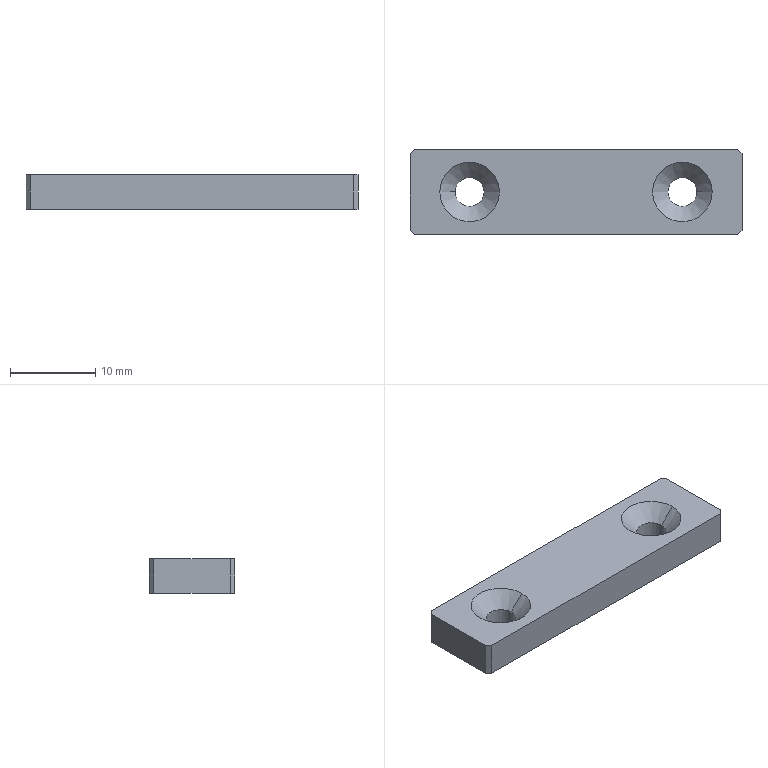Part | NX | features BREP 1 | 1 solid | 18 faces | box 39 x 10 x 4 mm | volume 1439 mm3 | plane 10 | cone 4 | cylinder 4 | commonest cylinder face diameters 3.4 x4
STEP:
#1=CARTESIAN_POINT('',(19.,-5.,4.));
#2=VERTEX_POINT('',#1);
#3=CARTESIAN_POINT('',(19.5,-4.5,4.));
#4=VERTEX_POINT('',#3);
#5=CARTESIAN_POINT('',(19.5,-4.5,4.));
#6=DIRECTION('',(0.7071,0.7071,0.));
#7=VECTOR('',#6,1000.);
#8=LINE('',#5,#7);
#9=EDGE_CURVE('',#2,#4,#8,.T.);
#10=ORIENTED_EDGE('',*,*,#9,.F.);
#11=CARTESIAN_POINT('',(19.,-5.,0.));
#12=VERTEX_POINT('',#11);
#13=CARTESIAN_POINT('',(19.,-5.,4.));
#14=DIRECTION('',(0.,0.,1.));
#15=VECTOR('',#14,1000.);
#16=LINE('',#13,#15);
#17=EDGE_CURVE('',#12,#2,#16,.T.);
#18=ORIENTED_EDGE('',*,*,#17,.F.);
#19=CARTESIAN_POINT('',(19.5,-4.5,0.));
#20=VERTEX_POINT('',#19);
#21=CARTESIAN_POINT('',(12.,-12.,0.));
#22=DIRECTION('',(-0.7071,-0.7071,0.));
#23=VECTOR('',#22,1000.);
#24=LINE('',#21,#23);
#25=EDGE_CURVE('',#20,#12,#24,.T.);
#26=ORIENTED_EDGE('',*,*,#25,.F.);
#27=CARTESIAN_POINT('',(19.5,-4.5,4.));
#28=DIRECTION('',(0.,0.,-1.));
#29=VECTOR('',#28,1000.);
#30=LINE('',#27,#29);
#31=EDGE_CURVE('',#4,#20,#30,.T.);
#32=ORIENTED_EDGE('',*,*,#31,.F.);
#33=EDGE_LOOP('',(#10,#18,#26,#32));
#34=FACE_BOUND('',#33,.T.);
#35=CARTESIAN_POINT('',(19.5,-4.5,4.));
#36=DIRECTION('',(-0.7071,0.7071,0.));
#37=DIRECTION('',(0.,0.,-1.));
#38=AXIS2_PLACEMENT_3D('',#35,#36,#37);
#39=PLANE('',#38);
#40=ADVANCED_FACE('',(#34),#39,.F.);
#41=CARTESIAN_POINT('',(19.5,4.5,4.));
#42=VERTEX_POINT('',#41);
#43=CARTESIAN_POINT('',(19.,5.,4.));
#44=VERTEX_POINT('',#43);
#45=CARTESIAN_POINT('',(19.,5.,4.));
#46=DIRECTION('',(-0.7071,0.7071,0.));
#47=VECTOR('',#46,1000.);
#48=LINE('',#45,#47);
#49=EDGE_CURVE('',#42,#44,#48,.T.);
#50=ORIENTED_EDGE('',*,*,#49,.F.);
#51=CARTESIAN_POINT('',(19.5,4.5,0.));
#52=VERTEX_POINT('',#51);
#53=CARTESIAN_POINT('',(19.5,4.5,4.));
#54=DIRECTION('',(0.,0.,1.));
#55=VECTOR('',#54,1000.);
#56=LINE('',#53,#55);
#57=EDGE_CURVE('',#52,#42,#56,.T.);
#58=ORIENTED_EDGE('',*,*,#57,.F.);
#59=CARTESIAN_POINT('',(19.,5.,0.));
#60=VERTEX_POINT('',#59);
#61=CARTESIAN_POINT('',(12.,12.,0.));
#62=DIRECTION('',(0.7071,-0.7071,0.));
#63=VECTOR('',#62,1000.);
#64=LINE('',#61,#63);
#65=EDGE_CURVE('',#60,#52,#64,.T.);
#66=ORIENTED_EDGE('',*,*,#65,.F.);
#67=CARTESIAN_POINT('',(19.,5.,4.));
#68=DIRECTION('',(0.,0.,-1.));
#69=VECTOR('',#68,1000.);
#70=LINE('',#67,#69);
#71=EDGE_CURVE('',#44,#60,#70,.T.);
#72=ORIENTED_EDGE('',*,*,#71,.F.);
#73=EDGE_LOOP('',(#50,#58,#66,#72));
#74=FACE_BOUND('',#73,.T.);
#75=CARTESIAN_POINT('',(19.,5.,4.));
#76=DIRECTION('',(-0.7071,-0.7071,0.));
#77=DIRECTION('',(0.,0.,-1.));
#78=AXIS2_PLACEMENT_3D('',#75,#76,#77);
#79=PLANE('',#78);
#80=ADVANCED_FACE('',(#74),#79,.F.);
#81=CARTESIAN_POINT('',(-19.,5.,4.));
#82=VERTEX_POINT('',#81);
#83=CARTESIAN_POINT('',(-19.5,4.5,4.));
#84=VERTEX_POINT('',#83);
#85=CARTESIAN_POINT('',(-19.5,4.5,4.));
#86=DIRECTION('',(-0.7071,-0.7071,0.));
#87=VECTOR('',#86,1000.);
#88=LINE('',#85,#87);
#89=EDGE_CURVE('',#82,#84,#88,.T.);
#90=ORIENTED_EDGE('',*,*,#89,.F.);
#91=CARTESIAN_POINT('',(-19.,5.,0.));
#92=VERTEX_POINT('',#91);
#93=CARTESIAN_POINT('',(-19.,5.,4.));
#94=DIRECTION('',(0.,0.,1.));
#95=VECTOR('',#94,1000.);
#96=LINE('',#93,#95);
#97=EDGE_CURVE('',#92,#82,#96,.T.);
#98=ORIENTED_EDGE('',*,*,#97,.F.);
#99=CARTESIAN_POINT('',(-19.5,4.5,0.));
#100=VERTEX_POINT('',#99);
#101=CARTESIAN_POINT('',(-12.,12.,0.));
#102=DIRECTION('',(0.7071,0.7071,0.));
#103=VECTOR('',#102,1000.);
#104=LINE('',#101,#103);
#105=EDGE_CURVE('',#100,#92,#104,.T.);
#106=ORIENTED_EDGE('',*,*,#105,.F.);
#107=CARTESIAN_POINT('',(-19.5,4.5,4.));
#108=DIRECTION('',(0.,0.,-1.));
#109=VECTOR('',#108,1000.);
#110=LINE('',#107,#109);
#111=EDGE_CURVE('',#84,#100,#110,.T.);
#112=ORIENTED_EDGE('',*,*,#111,.F.);
#113=EDGE_LOOP('',(#90,#98,#106,#112));
#114=FACE_BOUND('',#113,.T.);
#115=CARTESIAN_POINT('',(-19.5,4.5,4.));
#116=DIRECTION('',(0.7071,-0.7071,0.));
#117=DIRECTION('',(0.,0.,-1.));
#118=AXIS2_PLACEMENT_3D('',#115,#116,#117);
#119=PLANE('',#118);
#120=ADVANCED_FACE('',(#114),#119,.F.);
#121=CARTESIAN_POINT('',(-19.5,-4.5,4.));
#122=VERTEX_POINT('',#121);
#123=CARTESIAN_POINT('',(-19.,-5.,4.));
#124=VERTEX_POINT('',#123);
#125=CARTESIAN_POINT('',(-19.,-5.,4.));
#126=DIRECTION('',(0.7071,-0.7071,0.));
#127=VECTOR('',#126,1000.);
#128=LINE('',#125,#127);
#129=EDGE_CURVE('',#122,#124,#128,.T.);
#130=ORIENTED_EDGE('',*,*,#129,.F.);
#131=CARTESIAN_POINT('',(-19.5,-4.5,0.));
#132=VERTEX_POINT('',#131);
#133=CARTESIAN_POINT('',(-19.5,-4.5,4.));
#134=DIRECTION('',(0.,0.,1.));
#135=VECTOR('',#134,1000.);
#136=LINE('',#133,#135);
#137=EDGE_CURVE('',#132,#122,#136,.T.);
#138=ORIENTED_EDGE('',*,*,#137,.F.);
#139=CARTESIAN_POINT('',(-19.,-5.,0.));
#140=VERTEX_POINT('',#139);
#141=CARTESIAN_POINT('',(-12.,-12.,0.));
#142=DIRECTION('',(-0.7071,0.7071,0.));
#143=VECTOR('',#142,1000.);
#144=LINE('',#141,#143);
#145=EDGE_CURVE('',#140,#132,#144,.T.);
#146=ORIENTED_EDGE('',*,*,#145,.F.);
#147=CARTESIAN_POINT('',(-19.,-5.,4.));
#148=DIRECTION('',(0.,0.,-1.));
#149=VECTOR('',#148,1000.);
#150=LINE('',#147,#149);
#151=EDGE_CURVE('',#124,#140,#150,.T.);
#152=ORIENTED_EDGE('',*,*,#151,.F.);
#153=EDGE_LOOP('',(#130,#138,#146,#152));
#154=FACE_BOUND('',#153,.T.);
#155=CARTESIAN_POINT('',(-19.,-5.,4.));
#156=DIRECTION('',(0.7071,0.7071,0.));
#157=DIRECTION('',(0.,0.,-1.));
#158=AXIS2_PLACEMENT_3D('',#155,#156,#157);
#159=PLANE('',#158);
#160=ADVANCED_FACE('',(#154),#159,.F.);
#161=CARTESIAN_POINT('',(-16.,0.,4.));
#162=VERTEX_POINT('',#161);
#163=CARTESIAN_POINT('',(-14.2,0.,2.2));
#164=VERTEX_POINT('',#163);
#165=CARTESIAN_POINT('',(-16.,0.,4.));
#166=DIRECTION('',(-0.7071,0.,0.7071));
#167=VECTOR('',#166,1000.);
#168=LINE('',#165,#167);
#169=EDGE_CURVE('',#162,#164,#168,.F.);
#170=ORIENTED_EDGE('',*,*,#169,.T.);
#171=CARTESIAN_POINT('',(-10.8,0.,2.2));
#172=VERTEX_POINT('',#171);
#173=CARTESIAN_POINT('',(-12.5,0.,2.2));
#174=DIRECTION('',(0.,0.,1.));
#175=DIRECTION('',(1.,0.,0.));
#176=AXIS2_PLACEMENT_3D('',#173,#174,#175);
#177=CIRCLE('',#176,1.7);
#178=EDGE_CURVE('',#172,#164,#177,.T.);
#179=ORIENTED_EDGE('',*,*,#178,.F.);
#180=CARTESIAN_POINT('',(-9.,0.,4.));
#181=VERTEX_POINT('',#180);
#182=CARTESIAN_POINT('',(-9.,0.,4.));
#183=DIRECTION('',(0.7071,0.,0.7071));
#184=VECTOR('',#183,1000.);
#185=LINE('',#182,#184);
#186=EDGE_CURVE('',#181,#172,#185,.F.);
#187=ORIENTED_EDGE('',*,*,#186,.F.);
#188=CARTESIAN_POINT('',(-12.5,0.,4.));
#189=DIRECTION('',(0.,0.,1.));
#190=DIRECTION('',(1.,0.,0.));
#191=AXIS2_PLACEMENT_3D('',#188,#189,#190);
#192=CIRCLE('',#191,3.5);
#193=EDGE_CURVE('',#181,#162,#192,.T.);
#194=ORIENTED_EDGE('',*,*,#193,.T.);
#195=EDGE_LOOP('',(#170,#179,#187,#194));
#196=FACE_BOUND('',#195,.T.);
#197=CARTESIAN_POINT('',(-12.5,0.,4.));
#198=DIRECTION('',(0.,0.,1.));
#199=DIRECTION('',(1.,0.,0.));
#200=AXIS2_PLACEMENT_3D('',#197,#198,#199);
#201=CONICAL_SURFACE('',#200,3.5,0.7854);
#202=ADVANCED_FACE('',(#196),#201,.F.);
#203=CARTESIAN_POINT('',(-14.2,0.,0.));
#204=VERTEX_POINT('',#203);
#205=CARTESIAN_POINT('',(-14.2,0.,4.));
#206=DIRECTION('',(0.,0.,1.));
#207=VECTOR('',#206,1000.);
#208=LINE('',#205,#207);
#209=EDGE_CURVE('',#164,#204,#208,.F.);
#210=ORIENTED_EDGE('',*,*,#209,.T.);
#211=CARTESIAN_POINT('',(-10.8,0.,0.));
#212=VERTEX_POINT('',#211);
#213=CARTESIAN_POINT('',(-12.5,0.,0.));
#214=DIRECTION('',(0.,0.,-1.));
#215=DIRECTION('',(-1.,0.,0.));
#216=AXIS2_PLACEMENT_3D('',#213,#214,#215);
#217=CIRCLE('',#216,1.7);
#218=EDGE_CURVE('',#204,#212,#217,.T.);
#219=ORIENTED_EDGE('',*,*,#218,.T.);
#220=CARTESIAN_POINT('',(-10.8,0.,4.));
#221=DIRECTION('',(0.,0.,1.));
#222=VECTOR('',#221,1000.);
#223=LINE('',#220,#222);
#224=EDGE_CURVE('',#172,#212,#223,.F.);
#225=ORIENTED_EDGE('',*,*,#224,.F.);
#226=ORIENTED_EDGE('',*,*,#178,.T.);
#227=EDGE_LOOP('',(#210,#219,#225,#226));
#228=FACE_BOUND('',#227,.T.);
#229=CARTESIAN_POINT('',(-12.5,0.,4.));
#230=DIRECTION('',(0.,0.,1.));
#231=DIRECTION('',(1.,0.,0.));
#232=AXIS2_PLACEMENT_3D('',#229,#230,#231);
#233=CYLINDRICAL_SURFACE('',#232,1.7);
#234=ADVANCED_FACE('',(#228),#233,.F.);
#235=CARTESIAN_POINT('',(9.,0.,4.));
#236=VERTEX_POINT('',#235);
#237=CARTESIAN_POINT('',(10.8,0.,2.2));
#238=VERTEX_POINT('',#237);
#239=CARTESIAN_POINT('',(9.,0.,4.));
#240=DIRECTION('',(-0.7071,0.,0.7071));
#241=VECTOR('',#240,1000.);
#242=LINE('',#239,#241);
#243=EDGE_CURVE('',#236,#238,#242,.F.);
#244=ORIENTED_EDGE('',*,*,#243,.T.);
#245=CARTESIAN_POINT('',(14.2,0.,2.2));
#246=VERTEX_POINT('',#245);
#247=CARTESIAN_POINT('',(12.5,0.,2.2));
#248=DIRECTION('',(0.,0.,1.));
#249=DIRECTION('',(1.,0.,0.));
#250=AXIS2_PLACEMENT_3D('',#247,#248,#249);
#251=CIRCLE('',#250,1.7);
#252=EDGE_CURVE('',#246,#238,#251,.T.);
#253=ORIENTED_EDGE('',*,*,#252,.F.);
#254=CARTESIAN_POINT('',(16.,0.,4.));
#255=VERTEX_POINT('',#254);
#256=CARTESIAN_POINT('',(16.,0.,4.));
#257=DIRECTION('',(0.7071,0.,0.7071));
#258=VECTOR('',#257,1000.);
#259=LINE('',#256,#258);
#260=EDGE_CURVE('',#255,#246,#259,.F.);
#261=ORIENTED_EDGE('',*,*,#260,.F.);
#262=CARTESIAN_POINT('',(12.5,0.,4.));
#263=DIRECTION('',(0.,0.,1.));
#264=DIRECTION('',(1.,0.,0.));
#265=AXIS2_PLACEMENT_3D('',#262,#263,#264);
#266=CIRCLE('',#265,3.5);
#267=EDGE_CURVE('',#255,#236,#266,.T.);
#268=ORIENTED_EDGE('',*,*,#267,.T.);
#269=EDGE_LOOP('',(#244,#253,#261,#268));
#270=FACE_BOUND('',#269,.T.);
#271=CARTESIAN_POINT('',(12.5,0.,4.));
#272=DIRECTION('',(0.,0.,1.));
#273=DIRECTION('',(1.,0.,0.));
#274=AXIS2_PLACEMENT_3D('',#271,#272,#273);
#275=CONICAL_SURFACE('',#274,3.5,0.7854);
#276=ADVANCED_FACE('',(#270),#275,.F.);
#277=CARTESIAN_POINT('',(10.8,0.,0.));
#278=VERTEX_POINT('',#277);
#279=CARTESIAN_POINT('',(10.8,0.,4.));
#280=DIRECTION('',(0.,0.,1.));
#281=VECTOR('',#280,1000.);
#282=LINE('',#279,#281);
#283=EDGE_CURVE('',#238,#278,#282,.F.);
#284=ORIENTED_EDGE('',*,*,#283,.T.);
#285=CARTESIAN_POINT('',(14.2,0.,0.));
#286=VERTEX_POINT('',#285);
#287=CARTESIAN_POINT('',(12.5,0.,0.));
#288=DIRECTION('',(0.,0.,-1.));
#289=DIRECTION('',(-1.,0.,0.));
#290=AXIS2_PLACEMENT_3D('',#287,#288,#289);
#291=CIRCLE('',#290,1.7);
#292=EDGE_CURVE('',#278,#286,#291,.T.);
#293=ORIENTED_EDGE('',*,*,#292,.T.);
#294=CARTESIAN_POINT('',(14.2,0.,4.));
#295=DIRECTION('',(0.,0.,1.));
#296=VECTOR('',#295,1000.);
#297=LINE('',#294,#296);
#298=EDGE_CURVE('',#246,#286,#297,.F.);
#299=ORIENTED_EDGE('',*,*,#298,.F.);
#300=ORIENTED_EDGE('',*,*,#252,.T.);
#301=EDGE_LOOP('',(#284,#293,#299,#300));
#302=FACE_BOUND('',#301,.T.);
#303=CARTESIAN_POINT('',(12.5,0.,4.));
#304=DIRECTION('',(0.,0.,1.));
#305=DIRECTION('',(1.,0.,0.));
#306=AXIS2_PLACEMENT_3D('',#303,#304,#305);
#307=CYLINDRICAL_SURFACE('',#306,1.7);
#308=ADVANCED_FACE('',(#302),#307,.F.);
#309=CARTESIAN_POINT('',(-19.5,-5.,0.));
#310=DIRECTION('',(1.,0.,0.));
#311=VECTOR('',#310,1000.);
#312=LINE('',#309,#311);
#313=EDGE_CURVE('',#140,#12,#312,.T.);
#314=ORIENTED_EDGE('',*,*,#313,.F.);
#315=ORIENTED_EDGE('',*,*,#145,.T.);
#316=CARTESIAN_POINT('',(-19.5,-5.,0.));
#317=DIRECTION('',(0.,-1.,0.));
#318=VECTOR('',#317,1000.);
#319=LINE('',#316,#318);
#320=EDGE_CURVE('',#100,#132,#319,.T.);
#321=ORIENTED_EDGE('',*,*,#320,.F.);
#322=ORIENTED_EDGE('',*,*,#105,.T.);
#323=CARTESIAN_POINT('',(-19.5,5.,0.));
#324=DIRECTION('',(-1.,0.,0.));
#325=VECTOR('',#324,1000.);
#326=LINE('',#323,#325);
#327=EDGE_CURVE('',#60,#92,#326,.T.);
#328=ORIENTED_EDGE('',*,*,#327,.F.);
#329=ORIENTED_EDGE('',*,*,#65,.T.);
#330=CARTESIAN_POINT('',(19.5,-5.,0.));
#331=DIRECTION('',(0.,1.,0.));
#332=VECTOR('',#331,1000.);
#333=LINE('',#330,#332);
#334=EDGE_CURVE('',#20,#52,#333,.T.);
#335=ORIENTED_EDGE('',*,*,#334,.F.);
#336=ORIENTED_EDGE('',*,*,#25,.T.);
#337=EDGE_LOOP('',(#314,#315,#321,#322,#328,#329,#335,#336));
#338=FACE_BOUND('',#337,.T.);
#339=CARTESIAN_POINT('',(12.5,0.,0.));
#340=DIRECTION('',(0.,0.,-1.));
#341=DIRECTION('',(-1.,0.,0.));
#342=AXIS2_PLACEMENT_3D('',#339,#340,#341);
#343=CIRCLE('',#342,1.7);
#344=EDGE_CURVE('',#286,#278,#343,.T.);
#345=ORIENTED_EDGE('',*,*,#344,.F.);
#346=ORIENTED_EDGE('',*,*,#292,.F.);
#347=EDGE_LOOP('',(#345,#346));
#348=FACE_BOUND('',#347,.T.);
#349=CARTESIAN_POINT('',(-12.5,0.,0.));
#350=DIRECTION('',(0.,0.,-1.));
#351=DIRECTION('',(-1.,0.,0.));
#352=AXIS2_PLACEMENT_3D('',#349,#350,#351);
#353=CIRCLE('',#352,1.7);
#354=EDGE_CURVE('',#212,#204,#353,.T.);
#355=ORIENTED_EDGE('',*,*,#354,.F.);
#356=ORIENTED_EDGE('',*,*,#218,.F.);
#357=EDGE_LOOP('',(#355,#356));
#358=FACE_BOUND('',#357,.T.);
#359=CARTESIAN_POINT('',(0.,0.,0.));
#360=DIRECTION('',(0.,0.,-1.));
#361=DIRECTION('',(-1.,0.,0.));
#362=AXIS2_PLACEMENT_3D('',#359,#360,#361);
#363=PLANE('',#362);
#364=ADVANCED_FACE('',(#338,#348,#358),#363,.T.);
#365=CARTESIAN_POINT('',(-19.5,-5.,4.));
#366=DIRECTION('',(0.,-1.,0.));
#367=VECTOR('',#366,1000.);
#368=LINE('',#365,#367);
#369=EDGE_CURVE('',#84,#122,#368,.T.);
#370=ORIENTED_EDGE('',*,*,#369,.T.);
#371=ORIENTED_EDGE('',*,*,#129,.T.);
#372=CARTESIAN_POINT('',(-19.5,-5.,4.));
#373=DIRECTION('',(1.,0.,0.));
#374=VECTOR('',#373,1000.);
#375=LINE('',#372,#374);
#376=EDGE_CURVE('',#124,#2,#375,.T.);
#377=ORIENTED_EDGE('',*,*,#376,.T.);
#378=ORIENTED_EDGE('',*,*,#9,.T.);
#379=CARTESIAN_POINT('',(19.5,-5.,4.));
#380=DIRECTION('',(0.,1.,0.));
#381=VECTOR('',#380,1000.);
#382=LINE('',#379,#381);
#383=EDGE_CURVE('',#4,#42,#382,.T.);
#384=ORIENTED_EDGE('',*,*,#383,.T.);
#385=ORIENTED_EDGE('',*,*,#49,.T.);
#386=CARTESIAN_POINT('',(-19.5,5.,4.));
#387=DIRECTION('',(-1.,0.,0.));
#388=VECTOR('',#387,1000.);
#389=LINE('',#386,#388);
#390=EDGE_CURVE('',#44,#82,#389,.T.);
#391=ORIENTED_EDGE('',*,*,#390,.T.);
#392=ORIENTED_EDGE('',*,*,#89,.T.);
#393=EDGE_LOOP('',(#370,#371,#377,#378,#384,#385,#391,#392));
#394=FACE_BOUND('',#393,.T.);
#395=ORIENTED_EDGE('',*,*,#267,.F.);
#396=CARTESIAN_POINT('',(12.5,0.,4.));
#397=DIRECTION('',(0.,0.,1.));
#398=DIRECTION('',(1.,0.,0.));
#399=AXIS2_PLACEMENT_3D('',#396,#397,#398);
#400=CIRCLE('',#399,3.5);
#401=EDGE_CURVE('',#236,#255,#400,.T.);
#402=ORIENTED_EDGE('',*,*,#401,.F.);
#403=EDGE_LOOP('',(#395,#402));
#404=FACE_BOUND('',#403,.T.);
#405=ORIENTED_EDGE('',*,*,#193,.F.);
#406=CARTESIAN_POINT('',(-12.5,0.,4.));
#407=DIRECTION('',(0.,0.,1.));
#408=DIRECTION('',(1.,0.,0.));
#409=AXIS2_PLACEMENT_3D('',#406,#407,#408);
#410=CIRCLE('',#409,3.5);
#411=EDGE_CURVE('',#162,#181,#410,.T.);
#412=ORIENTED_EDGE('',*,*,#411,.F.);
#413=EDGE_LOOP('',(#405,#412));
#414=FACE_BOUND('',#413,.T.);
#415=CARTESIAN_POINT('',(0.,0.,4.));
#416=DIRECTION('',(0.,0.,-1.));
#417=DIRECTION('',(-1.,0.,0.));
#418=AXIS2_PLACEMENT_3D('',#415,#416,#417);
#419=PLANE('',#418);
#420=ADVANCED_FACE('',(#394,#404,#414),#419,.F.);
#421=ORIENTED_EDGE('',*,*,#376,.F.);
#422=ORIENTED_EDGE('',*,*,#151,.T.);
#423=ORIENTED_EDGE('',*,*,#313,.T.);
#424=ORIENTED_EDGE('',*,*,#17,.T.);
#425=EDGE_LOOP('',(#421,#422,#423,#424));
#426=FACE_BOUND('',#425,.T.);
#427=CARTESIAN_POINT('',(-19.5,-5.,4.));
#428=DIRECTION('',(0.,1.,0.));
#429=DIRECTION('',(0.,0.,1.));
#430=AXIS2_PLACEMENT_3D('',#427,#428,#429);
#431=PLANE('',#430);
#432=ADVANCED_FACE('',(#426),#431,.F.);
#433=ORIENTED_EDGE('',*,*,#320,.T.);
#434=ORIENTED_EDGE('',*,*,#137,.T.);
#435=ORIENTED_EDGE('',*,*,#369,.F.);
#436=ORIENTED_EDGE('',*,*,#111,.T.);
#437=EDGE_LOOP('',(#433,#434,#435,#436));
#438=FACE_BOUND('',#437,.T.);
#439=CARTESIAN_POINT('',(-19.5,-5.,4.));
#440=DIRECTION('',(1.,0.,0.));
#441=DIRECTION('',(0.,0.,-1.));
#442=AXIS2_PLACEMENT_3D('',#439,#440,#441);
#443=PLANE('',#442);
#444=ADVANCED_FACE('',(#438),#443,.F.);
#445=ORIENTED_EDGE('',*,*,#327,.T.);
#446=ORIENTED_EDGE('',*,*,#97,.T.);
#447=ORIENTED_EDGE('',*,*,#390,.F.);
#448=ORIENTED_EDGE('',*,*,#71,.T.);
#449=EDGE_LOOP('',(#445,#446,#447,#448));
#450=FACE_BOUND('',#449,.T.);
#451=CARTESIAN_POINT('',(-19.5,5.,4.));
#452=DIRECTION('',(0.,-1.,0.));
#453=DIRECTION('',(0.,0.,-1.));
#454=AXIS2_PLACEMENT_3D('',#451,#452,#453);
#455=PLANE('',#454);
#456=ADVANCED_FACE('',(#450),#455,.F.);
#457=ORIENTED_EDGE('',*,*,#334,.T.);
#458=ORIENTED_EDGE('',*,*,#57,.T.);
#459=ORIENTED_EDGE('',*,*,#383,.F.);
#460=ORIENTED_EDGE('',*,*,#31,.T.);
#461=EDGE_LOOP('',(#457,#458,#459,#460));
#462=FACE_BOUND('',#461,.T.);
#463=CARTESIAN_POINT('',(19.5,-5.,4.));
#464=DIRECTION('',(-1.,0.,0.));
#465=DIRECTION('',(0.,0.,1.));
#466=AXIS2_PLACEMENT_3D('',#463,#464,#465);
#467=PLANE('',#466);
#468=ADVANCED_FACE('',(#462),#467,.F.);
#469=ORIENTED_EDGE('',*,*,#344,.T.);
#470=ORIENTED_EDGE('',*,*,#283,.F.);
#471=CARTESIAN_POINT('',(12.5,0.,2.2));
#472=DIRECTION('',(0.,0.,1.));
#473=DIRECTION('',(1.,0.,0.));
#474=AXIS2_PLACEMENT_3D('',#471,#472,#473);
#475=CIRCLE('',#474,1.7);
#476=EDGE_CURVE('',#238,#246,#475,.T.);
#477=ORIENTED_EDGE('',*,*,#476,.T.);
#478=ORIENTED_EDGE('',*,*,#298,.T.);
#479=EDGE_LOOP('',(#469,#470,#477,#478));
#480=FACE_BOUND('',#479,.T.);
#481=CARTESIAN_POINT('',(12.5,0.,4.));
#482=DIRECTION('',(0.,0.,1.));
#483=DIRECTION('',(1.,0.,0.));
#484=AXIS2_PLACEMENT_3D('',#481,#482,#483);
#485=CYLINDRICAL_SURFACE('',#484,1.7);
#486=ADVANCED_FACE('',(#480),#485,.F.);
#487=ORIENTED_EDGE('',*,*,#476,.F.);
#488=ORIENTED_EDGE('',*,*,#243,.F.);
#489=ORIENTED_EDGE('',*,*,#401,.T.);
#490=ORIENTED_EDGE('',*,*,#260,.T.);
#491=EDGE_LOOP('',(#487,#488,#489,#490));
#492=FACE_BOUND('',#491,.T.);
#493=CARTESIAN_POINT('',(12.5,0.,4.));
#494=DIRECTION('',(0.,0.,1.));
#495=DIRECTION('',(1.,0.,0.));
#496=AXIS2_PLACEMENT_3D('',#493,#494,#495);
#497=CONICAL_SURFACE('',#496,3.5,0.7854);
#498=ADVANCED_FACE('',(#492),#497,.F.);
#499=ORIENTED_EDGE('',*,*,#354,.T.);
#500=ORIENTED_EDGE('',*,*,#209,.F.);
#501=CARTESIAN_POINT('',(-12.5,0.,2.2));
#502=DIRECTION('',(0.,0.,1.));
#503=DIRECTION('',(1.,0.,0.));
#504=AXIS2_PLACEMENT_3D('',#501,#502,#503);
#505=CIRCLE('',#504,1.7);
#506=EDGE_CURVE('',#164,#172,#505,.T.);
#507=ORIENTED_EDGE('',*,*,#506,.T.);
#508=ORIENTED_EDGE('',*,*,#224,.T.);
#509=EDGE_LOOP('',(#499,#500,#507,#508));
#510=FACE_BOUND('',#509,.T.);
#511=CARTESIAN_POINT('',(-12.5,0.,4.));
#512=DIRECTION('',(0.,0.,1.));
#513=DIRECTION('',(1.,0.,0.));
#514=AXIS2_PLACEMENT_3D('',#511,#512,#513);
#515=CYLINDRICAL_SURFACE('',#514,1.7);
#516=ADVANCED_FACE('',(#510),#515,.F.);
#517=ORIENTED_EDGE('',*,*,#506,.F.);
#518=ORIENTED_EDGE('',*,*,#169,.F.);
#519=ORIENTED_EDGE('',*,*,#411,.T.);
#520=ORIENTED_EDGE('',*,*,#186,.T.);
#521=EDGE_LOOP('',(#517,#518,#519,#520));
#522=FACE_BOUND('',#521,.T.);
#523=CARTESIAN_POINT('',(-12.5,0.,4.));
#524=DIRECTION('',(0.,0.,1.));
#525=DIRECTION('',(1.,0.,0.));
#526=AXIS2_PLACEMENT_3D('',#523,#524,#525);
#527=CONICAL_SURFACE('',#526,3.5,0.7854);
#528=ADVANCED_FACE('',(#522),#527,.F.);
#529=CLOSED_SHELL('',(#40,#80,#120,#160,#202,#234,#276,#308,#364,#420,#432,#444,#456,#468,#486,#498,#516,#528));
#530=MANIFOLD_SOLID_BREP('',#529);
#531=(LENGTH_UNIT()NAMED_UNIT(*)SI_UNIT(.MILLI.,.METRE.));
#532=UNCERTAINTY_MEASURE_WITH_UNIT(LENGTH_MEASURE(0.00001),#531,'','');
#533=(NAMED_UNIT(*)PLANE_ANGLE_UNIT()SI_UNIT($,.RADIAN.));
#534=(NAMED_UNIT(*)SI_UNIT($,.STERADIAN.)SOLID_ANGLE_UNIT());
#535=(GEOMETRIC_REPRESENTATION_CONTEXT(3)GLOBAL_UNCERTAINTY_ASSIGNED_CONTEXT((#532))GLOBAL_UNIT_ASSIGNED_CONTEXT((#531,#533,#534))REPRESENTATION_CONTEXT('',''));
#536=ADVANCED_BREP_SHAPE_REPRESENTATION('',(#530),#535);